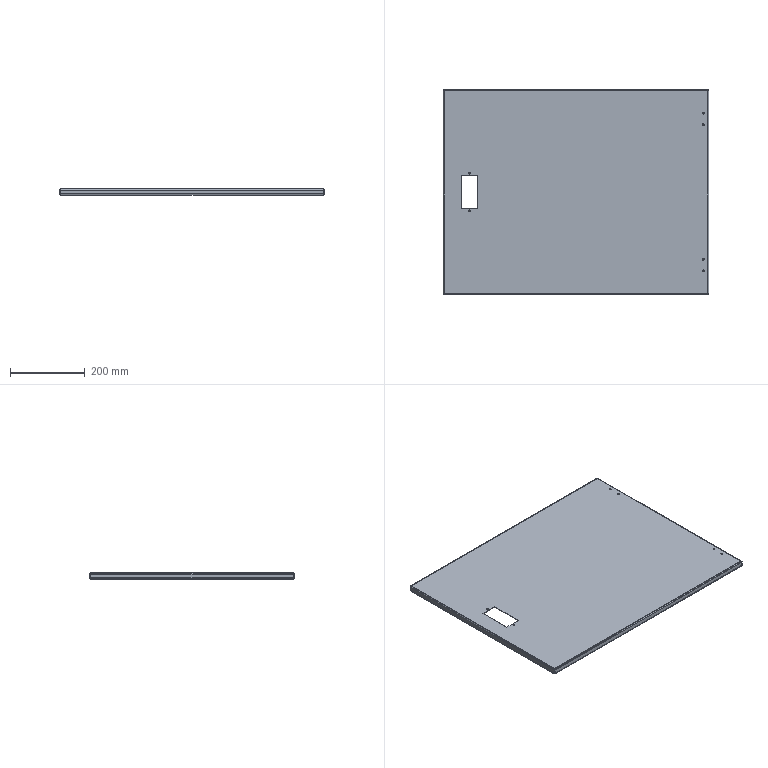Part | STEP file | QA-Door panel B-1 | 1 solid | 130 faces | box 708 x 546 x 16.5 mm | volume 666860 mm3 | plane 58 | spline 40 | cylinder 32 | commonest cylinder face diameters 3 x8 4.2 x8 6 x8 2 x4 4.5 x4